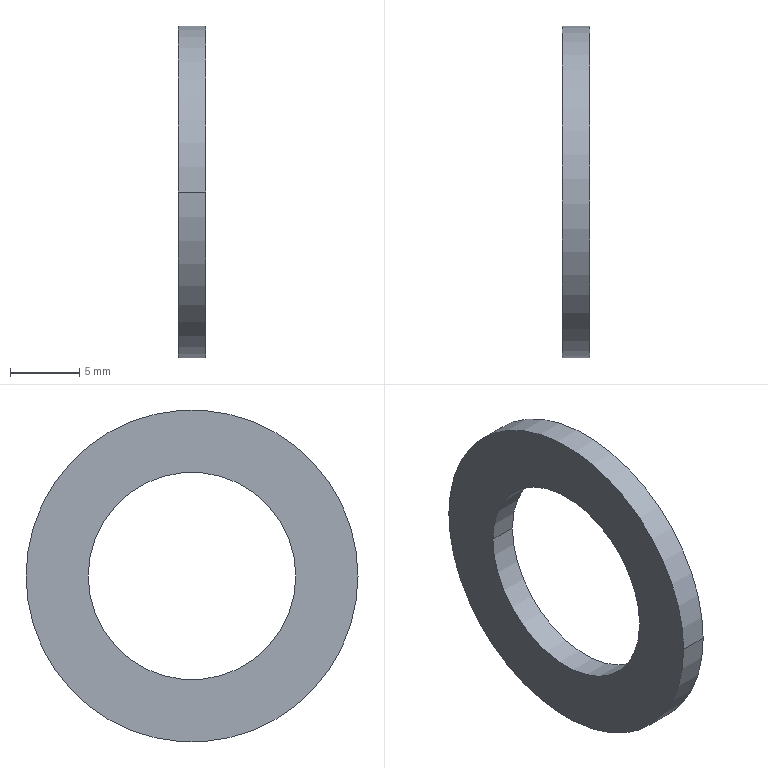Part | NX | features solid 2 | 1 solid | 6 faces | box 2 x 24 x 24 mm | volume 551.35 mm3 | cylinder 4 | plane 2 | commonest cylinder face diameters 15 x2 24 x2
STEP:
#1=CARTESIAN_POINT('',(164.1,-59.5,-954.));
#2=VERTEX_POINT('',#1);
#3=CARTESIAN_POINT('',(164.1,-83.5,-954.));
#4=VERTEX_POINT('',#3);
#5=CARTESIAN_POINT('',(164.1,-71.5,-954.));
#6=DIRECTION('',(1.,0.,0.));
#7=DIRECTION('',(0.,1.,0.));
#8=AXIS2_PLACEMENT_3D('',#5,#6,#7);
#9=CIRCLE('',#8,12.);
#10=EDGE_CURVE('',#2,#4,#9,.T.);
#11=ORIENTED_EDGE('',*,*,#10,.F.);
#12=CARTESIAN_POINT('',(164.1,-71.5,-954.));
#13=DIRECTION('',(1.,0.,0.));
#14=DIRECTION('',(0.,-1.,0.));
#15=AXIS2_PLACEMENT_3D('',#12,#13,#14);
#16=CIRCLE('',#15,12.);
#17=EDGE_CURVE('',#4,#2,#16,.T.);
#18=ORIENTED_EDGE('',*,*,#17,.F.);
#19=EDGE_LOOP('',(#11,#18));
#20=FACE_BOUND('',#19,.T.);
#21=CARTESIAN_POINT('',(164.1,-79.,-954.));
#22=VERTEX_POINT('',#21);
#23=CARTESIAN_POINT('',(164.1,-64.,-954.));
#24=VERTEX_POINT('',#23);
#25=CARTESIAN_POINT('',(164.1,-71.5,-954.));
#26=DIRECTION('',(-1.,0.,0.));
#27=DIRECTION('',(0.,-1.,0.));
#28=AXIS2_PLACEMENT_3D('',#25,#26,#27);
#29=CIRCLE('',#28,7.5);
#30=EDGE_CURVE('',#22,#24,#29,.T.);
#31=ORIENTED_EDGE('',*,*,#30,.F.);
#32=CARTESIAN_POINT('',(164.1,-71.5,-954.));
#33=DIRECTION('',(-1.,0.,0.));
#34=DIRECTION('',(0.,1.,0.));
#35=AXIS2_PLACEMENT_3D('',#32,#33,#34);
#36=CIRCLE('',#35,7.5);
#37=EDGE_CURVE('',#24,#22,#36,.T.);
#38=ORIENTED_EDGE('',*,*,#37,.F.);
#39=EDGE_LOOP('',(#31,#38));
#40=FACE_BOUND('',#39,.T.);
#41=CARTESIAN_POINT('',(164.1,-71.5,-954.));
#42=DIRECTION('',(1.,0.,0.));
#43=DIRECTION('',(0.,1.,0.));
#44=AXIS2_PLACEMENT_3D('',#41,#42,#43);
#45=PLANE('',#44);
#46=ADVANCED_FACE('',(#20,#40),#45,.F.);
#47=CARTESIAN_POINT('',(166.1,-59.5,-954.));
#48=VERTEX_POINT('',#47);
#49=CARTESIAN_POINT('',(166.1,-59.5,-954.));
#50=DIRECTION('',(-1.,0.,0.));
#51=VECTOR('',#50,1000.);
#52=LINE('',#49,#51);
#53=EDGE_CURVE('',#2,#48,#52,.F.);
#54=ORIENTED_EDGE('',*,*,#53,.T.);
#55=CARTESIAN_POINT('',(166.1,-83.5,-954.));
#56=VERTEX_POINT('',#55);
#57=CARTESIAN_POINT('',(166.1,-71.5,-954.));
#58=DIRECTION('',(-1.,0.,0.));
#59=DIRECTION('',(0.,1.,0.));
#60=AXIS2_PLACEMENT_3D('',#57,#58,#59);
#61=CIRCLE('',#60,12.);
#62=EDGE_CURVE('',#48,#56,#61,.T.);
#63=ORIENTED_EDGE('',*,*,#62,.T.);
#64=CARTESIAN_POINT('',(166.1,-83.5,-954.));
#65=DIRECTION('',(-1.,0.,0.));
#66=VECTOR('',#65,1000.);
#67=LINE('',#64,#66);
#68=EDGE_CURVE('',#56,#4,#67,.T.);
#69=ORIENTED_EDGE('',*,*,#68,.T.);
#70=ORIENTED_EDGE('',*,*,#17,.T.);
#71=EDGE_LOOP('',(#54,#63,#69,#70));
#72=FACE_BOUND('',#71,.T.);
#73=CARTESIAN_POINT('',(164.1,-71.5,-954.));
#74=DIRECTION('',(1.,0.,0.));
#75=DIRECTION('',(0.,1.,0.));
#76=AXIS2_PLACEMENT_3D('',#73,#74,#75);
#77=CYLINDRICAL_SURFACE('',#76,12.);
#78=ADVANCED_FACE('',(#72),#77,.T.);
#79=ORIENTED_EDGE('',*,*,#10,.T.);
#80=ORIENTED_EDGE('',*,*,#68,.F.);
#81=CARTESIAN_POINT('',(166.1,-71.5,-954.));
#82=DIRECTION('',(-1.,0.,0.));
#83=DIRECTION('',(0.,-1.,0.));
#84=AXIS2_PLACEMENT_3D('',#81,#82,#83);
#85=CIRCLE('',#84,12.);
#86=EDGE_CURVE('',#56,#48,#85,.T.);
#87=ORIENTED_EDGE('',*,*,#86,.T.);
#88=ORIENTED_EDGE('',*,*,#53,.F.);
#89=EDGE_LOOP('',(#79,#80,#87,#88));
#90=FACE_BOUND('',#89,.T.);
#91=CARTESIAN_POINT('',(164.1,-71.5,-954.));
#92=DIRECTION('',(1.,0.,0.));
#93=DIRECTION('',(0.,1.,0.));
#94=AXIS2_PLACEMENT_3D('',#91,#92,#93);
#95=CYLINDRICAL_SURFACE('',#94,12.);
#96=ADVANCED_FACE('',(#90),#95,.T.);
#97=ORIENTED_EDGE('',*,*,#86,.F.);
#98=ORIENTED_EDGE('',*,*,#62,.F.);
#99=EDGE_LOOP('',(#97,#98));
#100=FACE_BOUND('',#99,.T.);
#101=CARTESIAN_POINT('',(166.1,-79.,-954.));
#102=VERTEX_POINT('',#101);
#103=CARTESIAN_POINT('',(166.1,-64.,-954.));
#104=VERTEX_POINT('',#103);
#105=CARTESIAN_POINT('',(166.1,-71.5,-954.));
#106=DIRECTION('',(1.,0.,0.));
#107=DIRECTION('',(0.,-1.,0.));
#108=AXIS2_PLACEMENT_3D('',#105,#106,#107);
#109=CIRCLE('',#108,7.5);
#110=EDGE_CURVE('',#102,#104,#109,.T.);
#111=ORIENTED_EDGE('',*,*,#110,.F.);
#112=CARTESIAN_POINT('',(166.1,-71.5,-954.));
#113=DIRECTION('',(1.,0.,0.));
#114=DIRECTION('',(0.,1.,0.));
#115=AXIS2_PLACEMENT_3D('',#112,#113,#114);
#116=CIRCLE('',#115,7.5);
#117=EDGE_CURVE('',#104,#102,#116,.T.);
#118=ORIENTED_EDGE('',*,*,#117,.F.);
#119=EDGE_LOOP('',(#111,#118));
#120=FACE_BOUND('',#119,.T.);
#121=CARTESIAN_POINT('',(166.1,-71.5,-954.));
#122=DIRECTION('',(1.,0.,0.));
#123=DIRECTION('',(0.,1.,0.));
#124=AXIS2_PLACEMENT_3D('',#121,#122,#123);
#125=PLANE('',#124);
#126=ADVANCED_FACE('',(#100,#120),#125,.T.);
#127=CARTESIAN_POINT('',(166.1,-64.,-954.));
#128=DIRECTION('',(-1.,0.,0.));
#129=VECTOR('',#128,1000.);
#130=LINE('',#127,#129);
#131=EDGE_CURVE('',#24,#104,#130,.F.);
#132=ORIENTED_EDGE('',*,*,#131,.T.);
#133=ORIENTED_EDGE('',*,*,#117,.T.);
#134=CARTESIAN_POINT('',(166.1,-79.,-954.));
#135=DIRECTION('',(-1.,0.,0.));
#136=VECTOR('',#135,1000.);
#137=LINE('',#134,#136);
#138=EDGE_CURVE('',#102,#22,#137,.T.);
#139=ORIENTED_EDGE('',*,*,#138,.T.);
#140=ORIENTED_EDGE('',*,*,#30,.T.);
#141=EDGE_LOOP('',(#132,#133,#139,#140));
#142=FACE_BOUND('',#141,.T.);
#143=CARTESIAN_POINT('',(164.1,-71.5,-954.));
#144=DIRECTION('',(1.,0.,0.));
#145=DIRECTION('',(0.,1.,0.));
#146=AXIS2_PLACEMENT_3D('',#143,#144,#145);
#147=CYLINDRICAL_SURFACE('',#146,7.5);
#148=ADVANCED_FACE('',(#142),#147,.F.);
#149=ORIENTED_EDGE('',*,*,#37,.T.);
#150=ORIENTED_EDGE('',*,*,#138,.F.);
#151=ORIENTED_EDGE('',*,*,#110,.T.);
#152=ORIENTED_EDGE('',*,*,#131,.F.);
#153=EDGE_LOOP('',(#149,#150,#151,#152));
#154=FACE_BOUND('',#153,.T.);
#155=CARTESIAN_POINT('',(164.1,-71.5,-954.));
#156=DIRECTION('',(1.,0.,0.));
#157=DIRECTION('',(0.,1.,0.));
#158=AXIS2_PLACEMENT_3D('',#155,#156,#157);
#159=CYLINDRICAL_SURFACE('',#158,7.5);
#160=ADVANCED_FACE('',(#154),#159,.F.);
#161=CLOSED_SHELL('',(#46,#78,#96,#126,#148,#160));
#162=MANIFOLD_SOLID_BREP('',#161);
#163=(LENGTH_UNIT()NAMED_UNIT(*)SI_UNIT(.MILLI.,.METRE.));
#164=UNCERTAINTY_MEASURE_WITH_UNIT(LENGTH_MEASURE(0.00001),#163,'','');
#165=(NAMED_UNIT(*)PLANE_ANGLE_UNIT()SI_UNIT($,.RADIAN.));
#166=(NAMED_UNIT(*)SI_UNIT($,.STERADIAN.)SOLID_ANGLE_UNIT());
#167=(GEOMETRIC_REPRESENTATION_CONTEXT(3)GLOBAL_UNCERTAINTY_ASSIGNED_CONTEXT((#164))GLOBAL_UNIT_ASSIGNED_CONTEXT((#163,#165,#166))REPRESENTATION_CONTEXT('',''));
#168=ADVANCED_BREP_SHAPE_REPRESENTATION('',(#162),#167);